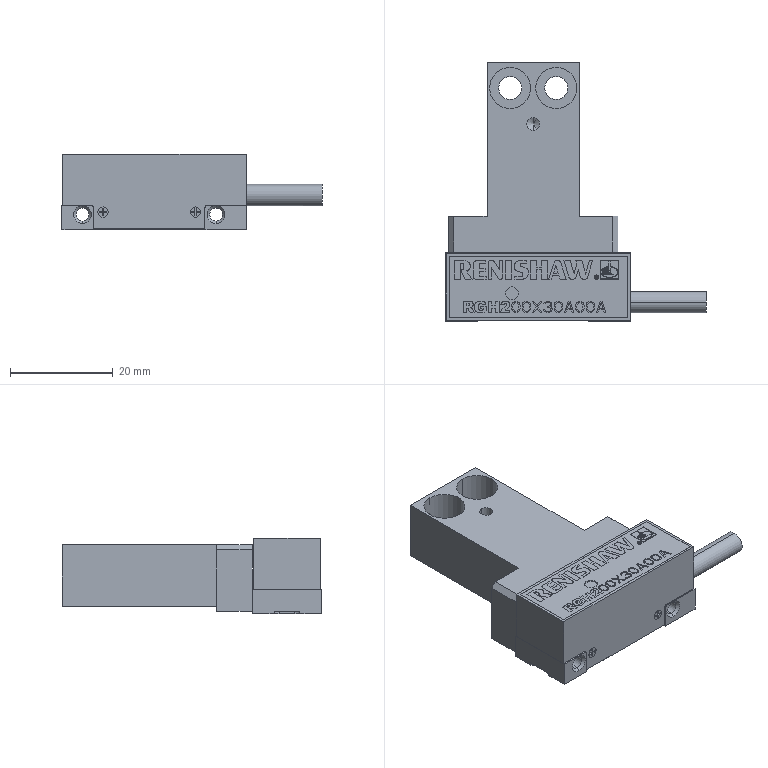Part | NX | features BREP 2 | 2 solids | 798 faces | box 50.65 x 50.5 x 14.8 mm | volume 15333 mm3 | plane 630 | spline 82 | cylinder 76 | cone 10 | commonest cylinder face diameters 2.5 x14 2 x6 1 x4 3.3 x4 4.5 x4 8 x4